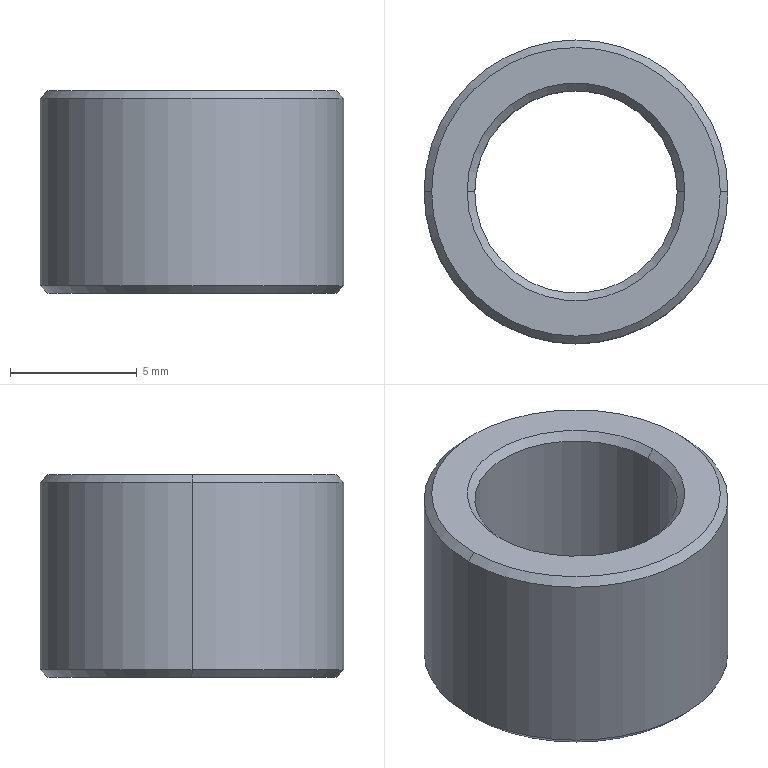Part | SolidWorks | features Chamfer 1, Extrusion 1 | 1 solid | 14 faces | box 12 x 12 x 8 mm | volume 497 mm3 | cone 8 | cylinder 4 | plane 2 | commonest cylinder face diameters 8 x2 12 x2
STEP:
#1=CARTESIAN_POINT('',(5.7,0.,4.));
#2=VERTEX_POINT('',#1);
#3=CARTESIAN_POINT('',(-5.7,0.,4.));
#4=VERTEX_POINT('',#3);
#5=CARTESIAN_POINT('',(0.,0.,4.));
#6=DIRECTION('',(0.,0.,1.));
#7=DIRECTION('',(1.,0.,0.));
#8=AXIS2_PLACEMENT_3D('',#5,#6,#7);
#9=CIRCLE('',#8,5.7);
#10=EDGE_CURVE('',#2,#4,#9,.T.);
#11=ORIENTED_EDGE('',*,*,#10,.F.);
#12=CARTESIAN_POINT('',(6.,0.,3.7));
#13=VERTEX_POINT('',#12);
#14=CARTESIAN_POINT('',(5.7,0.,4.));
#15=DIRECTION('',(0.7071,0.,-0.7071));
#16=VECTOR('',#15,1000.);
#17=LINE('',#14,#16);
#18=EDGE_CURVE('',#2,#13,#17,.T.);
#19=ORIENTED_EDGE('',*,*,#18,.T.);
#20=CARTESIAN_POINT('',(-6.,0.,3.7));
#21=VERTEX_POINT('',#20);
#22=CARTESIAN_POINT('',(0.,0.,3.7));
#23=DIRECTION('',(0.,0.,-1.));
#24=DIRECTION('',(1.,0.,0.));
#25=AXIS2_PLACEMENT_3D('',#22,#23,#24);
#26=CIRCLE('',#25,6.);
#27=EDGE_CURVE('',#21,#13,#26,.T.);
#28=ORIENTED_EDGE('',*,*,#27,.F.);
#29=CARTESIAN_POINT('',(-5.7,0.,4.));
#30=DIRECTION('',(-0.7071,0.,-0.7071));
#31=VECTOR('',#30,1000.);
#32=LINE('',#29,#31);
#33=EDGE_CURVE('',#4,#21,#32,.T.);
#34=ORIENTED_EDGE('',*,*,#33,.F.);
#35=EDGE_LOOP('',(#11,#19,#28,#34));
#36=FACE_OUTER_BOUND('',#35,.T.);
#37=CARTESIAN_POINT('',(0.,0.,4.));
#38=DIRECTION('',(0.,0.,-1.));
#39=DIRECTION('',(-1.,0.,0.));
#40=AXIS2_PLACEMENT_3D('',#37,#38,#39);
#41=CONICAL_SURFACE('',#40,5.7,0.7854);
#42=ADVANCED_FACE('',(#36),#41,.T.);
#43=CARTESIAN_POINT('',(-4.,0.,3.7));
#44=VERTEX_POINT('',#43);
#45=CARTESIAN_POINT('',(4.,0.,3.7));
#46=VERTEX_POINT('',#45);
#47=CARTESIAN_POINT('',(0.,0.,3.7));
#48=DIRECTION('',(0.,0.,1.));
#49=DIRECTION('',(1.,0.,0.));
#50=AXIS2_PLACEMENT_3D('',#47,#48,#49);
#51=CIRCLE('',#50,4.);
#52=EDGE_CURVE('',#44,#46,#51,.T.);
#53=ORIENTED_EDGE('',*,*,#52,.F.);
#54=CARTESIAN_POINT('',(-4.3,0.,4.));
#55=VERTEX_POINT('',#54);
#56=CARTESIAN_POINT('',(-4.,0.,3.7));
#57=DIRECTION('',(-0.7071,0.,0.7071));
#58=VECTOR('',#57,1000.);
#59=LINE('',#56,#58);
#60=EDGE_CURVE('',#44,#55,#59,.T.);
#61=ORIENTED_EDGE('',*,*,#60,.T.);
#62=CARTESIAN_POINT('',(4.3,0.,4.));
#63=VERTEX_POINT('',#62);
#64=CARTESIAN_POINT('',(0.,0.,4.));
#65=DIRECTION('',(0.,0.,-1.));
#66=DIRECTION('',(1.,0.,0.));
#67=AXIS2_PLACEMENT_3D('',#64,#65,#66);
#68=CIRCLE('',#67,4.3);
#69=EDGE_CURVE('',#63,#55,#68,.T.);
#70=ORIENTED_EDGE('',*,*,#69,.F.);
#71=CARTESIAN_POINT('',(4.,0.,3.7));
#72=DIRECTION('',(0.7071,0.,0.7071));
#73=VECTOR('',#72,1000.);
#74=LINE('',#71,#73);
#75=EDGE_CURVE('',#46,#63,#74,.T.);
#76=ORIENTED_EDGE('',*,*,#75,.F.);
#77=EDGE_LOOP('',(#53,#61,#70,#76));
#78=FACE_OUTER_BOUND('',#77,.T.);
#79=CARTESIAN_POINT('',(0.,0.,3.7));
#80=DIRECTION('',(0.,0.,1.));
#81=DIRECTION('',(1.,0.,0.));
#82=AXIS2_PLACEMENT_3D('',#79,#80,#81);
#83=CONICAL_SURFACE('',#82,4.,0.7854);
#84=ADVANCED_FACE('',(#78),#83,.F.);
#85=CARTESIAN_POINT('',(-5.7,0.,-4.));
#86=VERTEX_POINT('',#85);
#87=CARTESIAN_POINT('',(5.7,0.,-4.));
#88=VERTEX_POINT('',#87);
#89=CARTESIAN_POINT('',(0.,0.,-4.));
#90=DIRECTION('',(0.,0.,-1.));
#91=DIRECTION('',(1.,0.,0.));
#92=AXIS2_PLACEMENT_3D('',#89,#90,#91);
#93=CIRCLE('',#92,5.7);
#94=EDGE_CURVE('',#86,#88,#93,.T.);
#95=ORIENTED_EDGE('',*,*,#94,.F.);
#96=CARTESIAN_POINT('',(-6.,0.,-3.7));
#97=VERTEX_POINT('',#96);
#98=CARTESIAN_POINT('',(-6.,0.,-3.7));
#99=DIRECTION('',(-0.7071,0.,0.7071));
#100=VECTOR('',#99,1000.);
#101=LINE('',#98,#100);
#102=EDGE_CURVE('',#86,#97,#101,.T.);
#103=ORIENTED_EDGE('',*,*,#102,.T.);
#104=CARTESIAN_POINT('',(6.,0.,-3.7));
#105=VERTEX_POINT('',#104);
#106=CARTESIAN_POINT('',(0.,0.,-3.7));
#107=DIRECTION('',(0.,0.,1.));
#108=DIRECTION('',(1.,0.,0.));
#109=AXIS2_PLACEMENT_3D('',#106,#107,#108);
#110=CIRCLE('',#109,6.);
#111=EDGE_CURVE('',#105,#97,#110,.T.);
#112=ORIENTED_EDGE('',*,*,#111,.F.);
#113=CARTESIAN_POINT('',(6.,0.,-3.7));
#114=DIRECTION('',(0.7071,0.,0.7071));
#115=VECTOR('',#114,1000.);
#116=LINE('',#113,#115);
#117=EDGE_CURVE('',#88,#105,#116,.T.);
#118=ORIENTED_EDGE('',*,*,#117,.F.);
#119=EDGE_LOOP('',(#95,#103,#112,#118));
#120=FACE_OUTER_BOUND('',#119,.T.);
#121=CARTESIAN_POINT('',(0.,0.,-3.7));
#122=DIRECTION('',(0.,0.,1.));
#123=DIRECTION('',(1.,0.,0.));
#124=AXIS2_PLACEMENT_3D('',#121,#122,#123);
#125=CONICAL_SURFACE('',#124,6.,0.7854);
#126=ADVANCED_FACE('',(#120),#125,.T.);
#127=CARTESIAN_POINT('',(4.,0.,-3.7));
#128=VERTEX_POINT('',#127);
#129=CARTESIAN_POINT('',(-4.,0.,-3.7));
#130=VERTEX_POINT('',#129);
#131=CARTESIAN_POINT('',(0.,0.,-3.7));
#132=DIRECTION('',(0.,0.,-1.));
#133=DIRECTION('',(1.,0.,0.));
#134=AXIS2_PLACEMENT_3D('',#131,#132,#133);
#135=CIRCLE('',#134,4.);
#136=EDGE_CURVE('',#128,#130,#135,.T.);
#137=ORIENTED_EDGE('',*,*,#136,.F.);
#138=CARTESIAN_POINT('',(4.3,0.,-4.));
#139=VERTEX_POINT('',#138);
#140=CARTESIAN_POINT('',(4.3,0.,-4.));
#141=DIRECTION('',(0.7071,0.,-0.7071));
#142=VECTOR('',#141,1000.);
#143=LINE('',#140,#142);
#144=EDGE_CURVE('',#128,#139,#143,.T.);
#145=ORIENTED_EDGE('',*,*,#144,.T.);
#146=CARTESIAN_POINT('',(-4.3,0.,-4.));
#147=VERTEX_POINT('',#146);
#148=CARTESIAN_POINT('',(0.,0.,-4.));
#149=DIRECTION('',(0.,0.,1.));
#150=DIRECTION('',(1.,0.,0.));
#151=AXIS2_PLACEMENT_3D('',#148,#149,#150);
#152=CIRCLE('',#151,4.3);
#153=EDGE_CURVE('',#147,#139,#152,.T.);
#154=ORIENTED_EDGE('',*,*,#153,.F.);
#155=CARTESIAN_POINT('',(-4.3,0.,-4.));
#156=DIRECTION('',(-0.7071,0.,-0.7071));
#157=VECTOR('',#156,1000.);
#158=LINE('',#155,#157);
#159=EDGE_CURVE('',#130,#147,#158,.T.);
#160=ORIENTED_EDGE('',*,*,#159,.F.);
#161=EDGE_LOOP('',(#137,#145,#154,#160));
#162=FACE_OUTER_BOUND('',#161,.T.);
#163=CARTESIAN_POINT('',(0.,0.,-4.));
#164=DIRECTION('',(0.,0.,-1.));
#165=DIRECTION('',(-1.,0.,0.));
#166=AXIS2_PLACEMENT_3D('',#163,#164,#165);
#167=CONICAL_SURFACE('',#166,4.3,0.7854);
#168=ADVANCED_FACE('',(#162),#167,.F.);
#169=ORIENTED_EDGE('',*,*,#52,.T.);
#170=CARTESIAN_POINT('',(4.,0.,4.));
#171=DIRECTION('',(0.,0.,-1.));
#172=VECTOR('',#171,1000.);
#173=LINE('',#170,#172);
#174=EDGE_CURVE('',#46,#128,#173,.T.);
#175=ORIENTED_EDGE('',*,*,#174,.T.);
#176=ORIENTED_EDGE('',*,*,#136,.T.);
#177=CARTESIAN_POINT('',(-4.,0.,4.));
#178=DIRECTION('',(0.,0.,-1.));
#179=VECTOR('',#178,1000.);
#180=LINE('',#177,#179);
#181=EDGE_CURVE('',#44,#130,#180,.T.);
#182=ORIENTED_EDGE('',*,*,#181,.F.);
#183=EDGE_LOOP('',(#169,#175,#176,#182));
#184=FACE_OUTER_BOUND('',#183,.T.);
#185=CARTESIAN_POINT('',(0.,0.,4.));
#186=DIRECTION('',(0.,0.,-1.));
#187=DIRECTION('',(-1.,0.,0.));
#188=AXIS2_PLACEMENT_3D('',#185,#186,#187);
#189=CYLINDRICAL_SURFACE('',#188,4.);
#190=ADVANCED_FACE('',(#184),#189,.F.);
#191=ORIENTED_EDGE('',*,*,#27,.T.);
#192=CARTESIAN_POINT('',(6.,0.,4.));
#193=DIRECTION('',(0.,0.,-1.));
#194=VECTOR('',#193,1000.);
#195=LINE('',#192,#194);
#196=EDGE_CURVE('',#13,#105,#195,.T.);
#197=ORIENTED_EDGE('',*,*,#196,.T.);
#198=ORIENTED_EDGE('',*,*,#111,.T.);
#199=CARTESIAN_POINT('',(-6.,0.,4.));
#200=DIRECTION('',(0.,0.,-1.));
#201=VECTOR('',#200,1000.);
#202=LINE('',#199,#201);
#203=EDGE_CURVE('',#21,#97,#202,.T.);
#204=ORIENTED_EDGE('',*,*,#203,.F.);
#205=EDGE_LOOP('',(#191,#197,#198,#204));
#206=FACE_OUTER_BOUND('',#205,.T.);
#207=CARTESIAN_POINT('',(0.,0.,4.));
#208=DIRECTION('',(0.,0.,-1.));
#209=DIRECTION('',(-1.,0.,0.));
#210=AXIS2_PLACEMENT_3D('',#207,#208,#209);
#211=CYLINDRICAL_SURFACE('',#210,6.);
#212=ADVANCED_FACE('',(#206),#211,.T.);
#213=ORIENTED_EDGE('',*,*,#69,.T.);
#214=CARTESIAN_POINT('',(0.,0.,4.));
#215=DIRECTION('',(0.,0.,-1.));
#216=DIRECTION('',(1.,0.,0.));
#217=AXIS2_PLACEMENT_3D('',#214,#215,#216);
#218=CIRCLE('',#217,4.3);
#219=EDGE_CURVE('',#55,#63,#218,.T.);
#220=ORIENTED_EDGE('',*,*,#219,.T.);
#221=EDGE_LOOP('',(#213,#220));
#222=FACE_BOUND('',#221,.T.);
#223=CARTESIAN_POINT('',(0.,0.,4.));
#224=DIRECTION('',(0.,0.,1.));
#225=DIRECTION('',(1.,0.,0.));
#226=AXIS2_PLACEMENT_3D('',#223,#224,#225);
#227=CIRCLE('',#226,5.7);
#228=EDGE_CURVE('',#4,#2,#227,.T.);
#229=ORIENTED_EDGE('',*,*,#228,.T.);
#230=ORIENTED_EDGE('',*,*,#10,.T.);
#231=EDGE_LOOP('',(#229,#230));
#232=FACE_OUTER_BOUND('',#231,.T.);
#233=CARTESIAN_POINT('',(0.,0.,4.));
#234=DIRECTION('',(0.,0.,1.));
#235=DIRECTION('',(1.,0.,0.));
#236=AXIS2_PLACEMENT_3D('',#233,#234,#235);
#237=PLANE('',#236);
#238=ADVANCED_FACE('',(#222,#232),#237,.T.);
#239=ORIENTED_EDGE('',*,*,#153,.T.);
#240=CARTESIAN_POINT('',(0.,0.,-4.));
#241=DIRECTION('',(0.,0.,1.));
#242=DIRECTION('',(1.,0.,0.));
#243=AXIS2_PLACEMENT_3D('',#240,#241,#242);
#244=CIRCLE('',#243,4.3);
#245=EDGE_CURVE('',#139,#147,#244,.T.);
#246=ORIENTED_EDGE('',*,*,#245,.T.);
#247=EDGE_LOOP('',(#239,#246));
#248=FACE_BOUND('',#247,.T.);
#249=CARTESIAN_POINT('',(0.,0.,-4.));
#250=DIRECTION('',(0.,0.,-1.));
#251=DIRECTION('',(1.,0.,0.));
#252=AXIS2_PLACEMENT_3D('',#249,#250,#251);
#253=CIRCLE('',#252,5.7);
#254=EDGE_CURVE('',#88,#86,#253,.T.);
#255=ORIENTED_EDGE('',*,*,#254,.T.);
#256=ORIENTED_EDGE('',*,*,#94,.T.);
#257=EDGE_LOOP('',(#255,#256));
#258=FACE_OUTER_BOUND('',#257,.T.);
#259=CARTESIAN_POINT('',(0.,0.,-4.));
#260=DIRECTION('',(0.,0.,1.));
#261=DIRECTION('',(1.,0.,0.));
#262=AXIS2_PLACEMENT_3D('',#259,#260,#261);
#263=PLANE('',#262);
#264=ADVANCED_FACE('',(#248,#258),#263,.F.);
#265=ORIENTED_EDGE('',*,*,#196,.F.);
#266=CARTESIAN_POINT('',(0.,0.,3.7));
#267=DIRECTION('',(0.,0.,-1.));
#268=DIRECTION('',(1.,0.,0.));
#269=AXIS2_PLACEMENT_3D('',#266,#267,#268);
#270=CIRCLE('',#269,6.);
#271=EDGE_CURVE('',#13,#21,#270,.T.);
#272=ORIENTED_EDGE('',*,*,#271,.T.);
#273=ORIENTED_EDGE('',*,*,#203,.T.);
#274=CARTESIAN_POINT('',(0.,0.,-3.7));
#275=DIRECTION('',(0.,0.,1.));
#276=DIRECTION('',(1.,0.,0.));
#277=AXIS2_PLACEMENT_3D('',#274,#275,#276);
#278=CIRCLE('',#277,6.);
#279=EDGE_CURVE('',#97,#105,#278,.T.);
#280=ORIENTED_EDGE('',*,*,#279,.T.);
#281=EDGE_LOOP('',(#265,#272,#273,#280));
#282=FACE_OUTER_BOUND('',#281,.T.);
#283=CARTESIAN_POINT('',(0.,0.,4.));
#284=DIRECTION('',(0.,0.,-1.));
#285=DIRECTION('',(-1.,0.,0.));
#286=AXIS2_PLACEMENT_3D('',#283,#284,#285);
#287=CYLINDRICAL_SURFACE('',#286,6.);
#288=ADVANCED_FACE('',(#282),#287,.T.);
#289=ORIENTED_EDGE('',*,*,#174,.F.);
#290=CARTESIAN_POINT('',(0.,0.,3.7));
#291=DIRECTION('',(0.,0.,1.));
#292=DIRECTION('',(1.,0.,0.));
#293=AXIS2_PLACEMENT_3D('',#290,#291,#292);
#294=CIRCLE('',#293,4.);
#295=EDGE_CURVE('',#46,#44,#294,.T.);
#296=ORIENTED_EDGE('',*,*,#295,.T.);
#297=ORIENTED_EDGE('',*,*,#181,.T.);
#298=CARTESIAN_POINT('',(0.,0.,-3.7));
#299=DIRECTION('',(0.,0.,-1.));
#300=DIRECTION('',(1.,0.,0.));
#301=AXIS2_PLACEMENT_3D('',#298,#299,#300);
#302=CIRCLE('',#301,4.);
#303=EDGE_CURVE('',#130,#128,#302,.T.);
#304=ORIENTED_EDGE('',*,*,#303,.T.);
#305=EDGE_LOOP('',(#289,#296,#297,#304));
#306=FACE_OUTER_BOUND('',#305,.T.);
#307=CARTESIAN_POINT('',(0.,0.,4.));
#308=DIRECTION('',(0.,0.,-1.));
#309=DIRECTION('',(-1.,0.,0.));
#310=AXIS2_PLACEMENT_3D('',#307,#308,#309);
#311=CYLINDRICAL_SURFACE('',#310,4.);
#312=ADVANCED_FACE('',(#306),#311,.F.);
#313=ORIENTED_EDGE('',*,*,#144,.F.);
#314=ORIENTED_EDGE('',*,*,#303,.F.);
#315=ORIENTED_EDGE('',*,*,#159,.T.);
#316=ORIENTED_EDGE('',*,*,#245,.F.);
#317=EDGE_LOOP('',(#313,#314,#315,#316));
#318=FACE_OUTER_BOUND('',#317,.T.);
#319=CARTESIAN_POINT('',(0.,0.,-4.));
#320=DIRECTION('',(0.,0.,-1.));
#321=DIRECTION('',(-1.,0.,0.));
#322=AXIS2_PLACEMENT_3D('',#319,#320,#321);
#323=CONICAL_SURFACE('',#322,4.3,0.7854);
#324=ADVANCED_FACE('',(#318),#323,.F.);
#325=ORIENTED_EDGE('',*,*,#102,.F.);
#326=ORIENTED_EDGE('',*,*,#254,.F.);
#327=ORIENTED_EDGE('',*,*,#117,.T.);
#328=ORIENTED_EDGE('',*,*,#279,.F.);
#329=EDGE_LOOP('',(#325,#326,#327,#328));
#330=FACE_OUTER_BOUND('',#329,.T.);
#331=CARTESIAN_POINT('',(0.,0.,-3.7));
#332=DIRECTION('',(0.,0.,1.));
#333=DIRECTION('',(1.,0.,0.));
#334=AXIS2_PLACEMENT_3D('',#331,#332,#333);
#335=CONICAL_SURFACE('',#334,6.,0.7854);
#336=ADVANCED_FACE('',(#330),#335,.T.);
#337=ORIENTED_EDGE('',*,*,#60,.F.);
#338=ORIENTED_EDGE('',*,*,#295,.F.);
#339=ORIENTED_EDGE('',*,*,#75,.T.);
#340=ORIENTED_EDGE('',*,*,#219,.F.);
#341=EDGE_LOOP('',(#337,#338,#339,#340));
#342=FACE_OUTER_BOUND('',#341,.T.);
#343=CARTESIAN_POINT('',(0.,0.,3.7));
#344=DIRECTION('',(0.,0.,1.));
#345=DIRECTION('',(1.,0.,0.));
#346=AXIS2_PLACEMENT_3D('',#343,#344,#345);
#347=CONICAL_SURFACE('',#346,4.,0.7854);
#348=ADVANCED_FACE('',(#342),#347,.F.);
#349=ORIENTED_EDGE('',*,*,#18,.F.);
#350=ORIENTED_EDGE('',*,*,#228,.F.);
#351=ORIENTED_EDGE('',*,*,#33,.T.);
#352=ORIENTED_EDGE('',*,*,#271,.F.);
#353=EDGE_LOOP('',(#349,#350,#351,#352));
#354=FACE_OUTER_BOUND('',#353,.T.);
#355=CARTESIAN_POINT('',(0.,0.,4.));
#356=DIRECTION('',(0.,0.,-1.));
#357=DIRECTION('',(-1.,0.,0.));
#358=AXIS2_PLACEMENT_3D('',#355,#356,#357);
#359=CONICAL_SURFACE('',#358,5.7,0.7854);
#360=ADVANCED_FACE('',(#354),#359,.T.);
#361=CLOSED_SHELL('',(#42,#84,#126,#168,#190,#212,#238,#264,#288,#312,#324,#336,#348,#360));
#362=MANIFOLD_SOLID_BREP('',#361);
#363=CARTESIAN_POINT('',(0.,0.,0.));
#364=DIRECTION('',(0.,0.,1.));
#365=DIRECTION('',(1.,0.,0.));
#366=AXIS2_PLACEMENT_3D('',#363,#364,#365);
#367=(LENGTH_UNIT()NAMED_UNIT(*)SI_UNIT(.MILLI.,.METRE.));
#368=UNCERTAINTY_MEASURE_WITH_UNIT(LENGTH_MEASURE(0.00001),#367,'','');
#369=(NAMED_UNIT(*)PLANE_ANGLE_UNIT()SI_UNIT($,.RADIAN.));
#370=(NAMED_UNIT(*)SI_UNIT($,.STERADIAN.)SOLID_ANGLE_UNIT());
#371=(GEOMETRIC_REPRESENTATION_CONTEXT(3)GLOBAL_UNCERTAINTY_ASSIGNED_CONTEXT((#368))GLOBAL_UNIT_ASSIGNED_CONTEXT((#367,#369,#370))REPRESENTATION_CONTEXT('',''));
#372=ADVANCED_BREP_SHAPE_REPRESENTATION('',(#362,#366),#371);